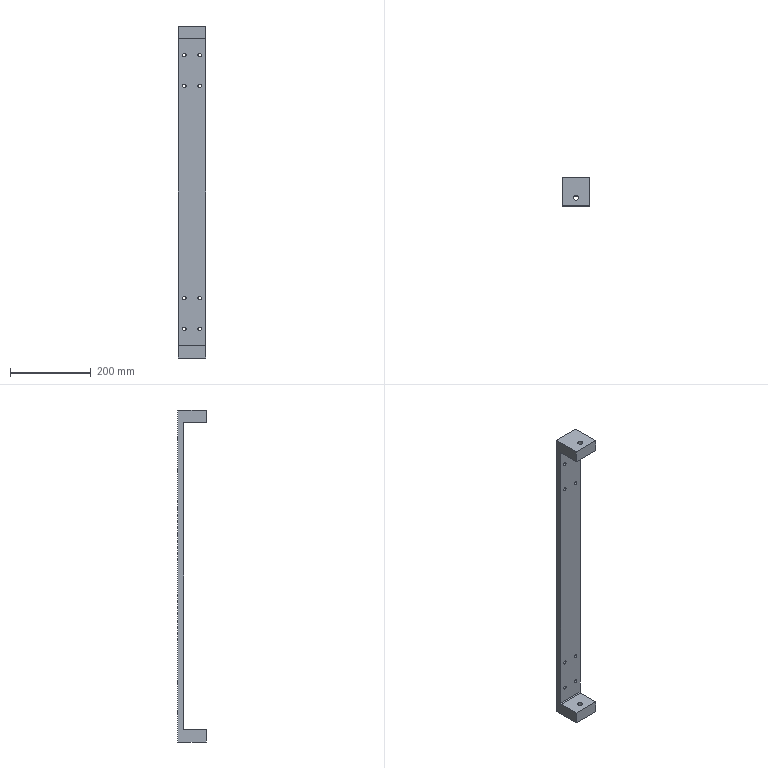Part | STEP file | Front link plate | 1 solid | 32 faces | box 68 x 70 x 820 mm | volume 1047322 mm3 | cylinder 22 | plane 10 | commonest cylinder face diameters 8.5 x16 12 x4 4 x2